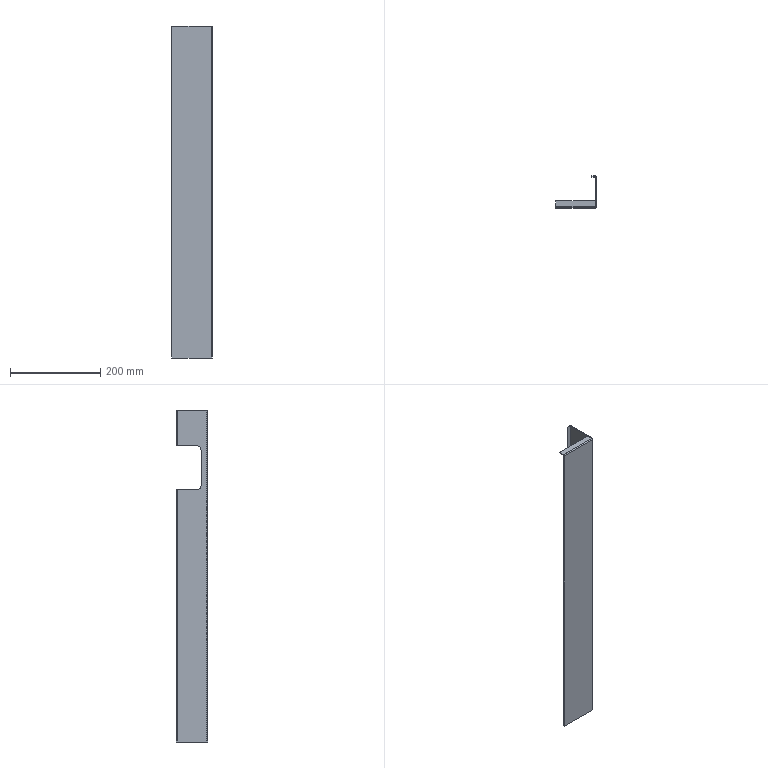Part | STEP file | Trunking 2 | 1 solid | 31 faces | box 90 x 70 x 735 mm | volume 175454 mm3 | plane 21 | cylinder 10 | commonest cylinder face diameters 1 x4 4 x4 20 x2
STEP:
#1=CARTESIAN_POINT('',(72.026,-9.818,0.));
#2=VERTEX_POINT('',#1);
#3=CARTESIAN_POINT('',(72.026,-9.818,733.));
#4=VERTEX_POINT('',#3);
#5=CARTESIAN_POINT('',(72.026,-9.818,735.));
#6=DIRECTION('',(0.,0.,1.));
#7=VECTOR('',#6,1000.);
#8=LINE('',#5,#7);
#9=EDGE_CURVE('',#2,#4,#8,.T.);
#10=ORIENTED_EDGE('',*,*,#9,.F.);
#11=CARTESIAN_POINT('',(-15.974,-9.818,0.));
#12=VERTEX_POINT('',#11);
#13=CARTESIAN_POINT('',(74.026,-9.818,0.));
#14=DIRECTION('',(1.,0.,0.));
#15=VECTOR('',#14,1000.);
#16=LINE('',#13,#15);
#17=EDGE_CURVE('',#12,#2,#16,.T.);
#18=ORIENTED_EDGE('',*,*,#17,.F.);
#19=CARTESIAN_POINT('',(-15.974,-9.818,733.));
#20=VERTEX_POINT('',#19);
#21=CARTESIAN_POINT('',(-15.974,-9.818,735.));
#22=DIRECTION('',(0.,0.,-1.));
#23=VECTOR('',#22,1000.);
#24=LINE('',#21,#23);
#25=EDGE_CURVE('',#20,#12,#24,.T.);
#26=ORIENTED_EDGE('',*,*,#25,.F.);
#27=CARTESIAN_POINT('',(74.026,-9.818,733.));
#28=DIRECTION('',(-1.,0.,0.));
#29=VECTOR('',#28,1000.);
#30=LINE('',#27,#29);
#31=EDGE_CURVE('',#4,#20,#30,.T.);
#32=ORIENTED_EDGE('',*,*,#31,.F.);
#33=EDGE_LOOP('',(#10,#18,#26,#32));
#34=FACE_OUTER_BOUND('',#33,.T.);
#35=CARTESIAN_POINT('',(74.026,-9.818,735.));
#36=DIRECTION('',(0.,-1.,0.));
#37=DIRECTION('',(1.,0.,0.));
#38=AXIS2_PLACEMENT_3D('',#35,#36,#37);
#39=PLANE('',#38);
#40=ADVANCED_FACE('',(#34),#39,.F.);
#41=CARTESIAN_POINT('',(-15.974,-9.318,733.5));
#42=VERTEX_POINT('',#41);
#43=CARTESIAN_POINT('',(-15.974,-9.318,733.));
#44=DIRECTION('',(1.,0.,0.));
#45=DIRECTION('',(0.,0.,-1.));
#46=AXIS2_PLACEMENT_3D('',#43,#44,#45);
#47=CIRCLE('',#46,0.5);
#48=EDGE_CURVE('',#42,#20,#47,.T.);
#49=ORIENTED_EDGE('',*,*,#48,.F.);
#50=CARTESIAN_POINT('',(72.026,-9.318,733.5));
#51=VERTEX_POINT('',#50);
#52=CARTESIAN_POINT('',(72.026,-9.318,733.5));
#53=DIRECTION('',(-1.,0.,0.));
#54=VECTOR('',#53,1000.);
#55=LINE('',#52,#54);
#56=EDGE_CURVE('',#51,#42,#55,.T.);
#57=ORIENTED_EDGE('',*,*,#56,.F.);
#58=CARTESIAN_POINT('',(72.026,-9.318,733.));
#59=DIRECTION('',(1.,0.,0.));
#60=DIRECTION('',(0.,0.,-1.));
#61=AXIS2_PLACEMENT_3D('',#58,#59,#60);
#62=CIRCLE('',#61,0.5);
#63=EDGE_CURVE('',#51,#4,#62,.T.);
#64=ORIENTED_EDGE('',*,*,#63,.T.);
#65=ORIENTED_EDGE('',*,*,#31,.T.);
#66=EDGE_LOOP('',(#49,#57,#64,#65));
#67=FACE_OUTER_BOUND('',#66,.T.);
#68=CARTESIAN_POINT('',(72.026,-9.318,733.));
#69=DIRECTION('',(1.,0.,0.));
#70=DIRECTION('',(0.,0.,-1.));
#71=AXIS2_PLACEMENT_3D('',#68,#69,#70);
#72=CYLINDRICAL_SURFACE('',#71,0.5);
#73=ADVANCED_FACE('',(#67),#72,.F.);
#74=ORIENTED_EDGE('',*,*,#9,.T.);
#75=CARTESIAN_POINT('',(72.026,-9.818,734.936));
#76=VERTEX_POINT('',#75);
#77=CARTESIAN_POINT('',(72.026,-9.818,735.));
#78=DIRECTION('',(0.,0.,-1.));
#79=VECTOR('',#78,1000.);
#80=LINE('',#77,#79);
#81=EDGE_CURVE('',#76,#4,#80,.T.);
#82=ORIENTED_EDGE('',*,*,#81,.F.);
#83=CARTESIAN_POINT('',(72.026,-9.818,735.));
#84=VERTEX_POINT('',#83);
#85=CARTESIAN_POINT('',(72.026,-9.818,735.));
#86=DIRECTION('',(0.,0.,-1.));
#87=VECTOR('',#86,1000.);
#88=LINE('',#85,#87);
#89=EDGE_CURVE('',#84,#76,#88,.T.);
#90=ORIENTED_EDGE('',*,*,#89,.F.);
#91=CARTESIAN_POINT('',(72.526,-9.318,735.));
#92=VERTEX_POINT('',#91);
#93=CARTESIAN_POINT('',(72.026,-9.318,735.));
#94=DIRECTION('',(0.,0.,-1.));
#95=DIRECTION('',(-1.,0.,0.));
#96=AXIS2_PLACEMENT_3D('',#93,#94,#95);
#97=CIRCLE('',#96,0.5);
#98=EDGE_CURVE('',#92,#84,#97,.T.);
#99=ORIENTED_EDGE('',*,*,#98,.F.);
#100=CARTESIAN_POINT('',(72.526,-9.318,0.));
#101=VERTEX_POINT('',#100);
#102=CARTESIAN_POINT('',(72.526,-9.318,735.));
#103=DIRECTION('',(0.,0.,1.));
#104=VECTOR('',#103,1000.);
#105=LINE('',#102,#104);
#106=EDGE_CURVE('',#101,#92,#105,.T.);
#107=ORIENTED_EDGE('',*,*,#106,.F.);
#108=CARTESIAN_POINT('',(72.026,-9.318,0.));
#109=DIRECTION('',(0.,0.,1.));
#110=DIRECTION('',(-1.,0.,0.));
#111=AXIS2_PLACEMENT_3D('',#108,#109,#110);
#112=CIRCLE('',#111,0.5);
#113=EDGE_CURVE('',#2,#101,#112,.T.);
#114=ORIENTED_EDGE('',*,*,#113,.F.);
#115=EDGE_LOOP('',(#74,#82,#90,#99,#107,#114));
#116=FACE_OUTER_BOUND('',#115,.T.);
#117=CARTESIAN_POINT('',(72.026,-9.318,735.));
#118=DIRECTION('',(0.,0.,-1.));
#119=DIRECTION('',(-1.,0.,0.));
#120=AXIS2_PLACEMENT_3D('',#117,#118,#119);
#121=CYLINDRICAL_SURFACE('',#120,0.5);
#122=ADVANCED_FACE('',(#116),#121,.F.);
#123=ORIENTED_EDGE('',*,*,#17,.T.);
#124=ORIENTED_EDGE('',*,*,#113,.T.);
#125=CARTESIAN_POINT('',(72.526,56.682,0.));
#126=VERTEX_POINT('',#125);
#127=CARTESIAN_POINT('',(72.526,58.682,0.));
#128=DIRECTION('',(0.,1.,0.));
#129=VECTOR('',#128,1000.);
#130=LINE('',#127,#129);
#131=EDGE_CURVE('',#101,#126,#130,.T.);
#132=ORIENTED_EDGE('',*,*,#131,.T.);
#133=CARTESIAN_POINT('',(72.026,57.182,0.));
#134=VERTEX_POINT('',#133);
#135=CARTESIAN_POINT('',(72.026,56.682,0.));
#136=DIRECTION('',(0.,0.,-1.));
#137=DIRECTION('',(-1.,0.,0.));
#138=AXIS2_PLACEMENT_3D('',#135,#136,#137);
#139=CIRCLE('',#138,0.5);
#140=EDGE_CURVE('',#134,#126,#139,.T.);
#141=ORIENTED_EDGE('',*,*,#140,.F.);
#142=CARTESIAN_POINT('',(64.026,57.182,0.));
#143=VERTEX_POINT('',#142);
#144=CARTESIAN_POINT('',(0.,57.182,0.));
#145=DIRECTION('',(1.,0.,0.));
#146=VECTOR('',#145,1000.);
#147=LINE('',#144,#146);
#148=EDGE_CURVE('',#143,#134,#147,.T.);
#149=ORIENTED_EDGE('',*,*,#148,.F.);
#150=CARTESIAN_POINT('',(64.026,58.682,0.));
#151=VERTEX_POINT('',#150);
#152=CARTESIAN_POINT('',(64.026,58.682,0.));
#153=DIRECTION('',(0.,1.,0.));
#154=VECTOR('',#153,1000.);
#155=LINE('',#152,#154);
#156=EDGE_CURVE('',#143,#151,#155,.T.);
#157=ORIENTED_EDGE('',*,*,#156,.T.);
#158=CARTESIAN_POINT('',(72.026,58.682,0.));
#159=VERTEX_POINT('',#158);
#160=CARTESIAN_POINT('',(0.,58.682,0.));
#161=DIRECTION('',(1.,0.,0.));
#162=VECTOR('',#161,1000.);
#163=LINE('',#160,#162);
#164=EDGE_CURVE('',#151,#159,#163,.T.);
#165=ORIENTED_EDGE('',*,*,#164,.T.);
#166=CARTESIAN_POINT('',(74.026,56.682,0.));
#167=VERTEX_POINT('',#166);
#168=CARTESIAN_POINT('',(72.026,56.682,0.));
#169=DIRECTION('',(0.,0.,1.));
#170=DIRECTION('',(-1.,0.,0.));
#171=AXIS2_PLACEMENT_3D('',#168,#169,#170);
#172=CIRCLE('',#171,2.);
#173=EDGE_CURVE('',#167,#159,#172,.T.);
#174=ORIENTED_EDGE('',*,*,#173,.F.);
#175=CARTESIAN_POINT('',(74.026,-9.318,0.));
#176=VERTEX_POINT('',#175);
#177=CARTESIAN_POINT('',(74.026,-9.818,0.));
#178=DIRECTION('',(0.,-1.,0.));
#179=VECTOR('',#178,1000.);
#180=LINE('',#177,#179);
#181=EDGE_CURVE('',#167,#176,#180,.T.);
#182=ORIENTED_EDGE('',*,*,#181,.T.);
#183=CARTESIAN_POINT('',(72.026,-11.318,0.));
#184=VERTEX_POINT('',#183);
#185=CARTESIAN_POINT('',(72.026,-9.318,0.));
#186=DIRECTION('',(0.,0.,1.));
#187=DIRECTION('',(-1.,0.,0.));
#188=AXIS2_PLACEMENT_3D('',#185,#186,#187);
#189=CIRCLE('',#188,2.);
#190=EDGE_CURVE('',#184,#176,#189,.T.);
#191=ORIENTED_EDGE('',*,*,#190,.F.);
#192=CARTESIAN_POINT('',(-15.974,-11.318,0.));
#193=VERTEX_POINT('',#192);
#194=CARTESIAN_POINT('',(72.026,-11.318,0.));
#195=DIRECTION('',(1.,0.,0.));
#196=VECTOR('',#195,1000.);
#197=LINE('',#194,#196);
#198=EDGE_CURVE('',#193,#184,#197,.T.);
#199=ORIENTED_EDGE('',*,*,#198,.F.);
#200=CARTESIAN_POINT('',(-15.974,-9.318,0.));
#201=DIRECTION('',(0.,-1.,0.));
#202=VECTOR('',#201,1000.);
#203=LINE('',#200,#202);
#204=EDGE_CURVE('',#12,#193,#203,.T.);
#205=ORIENTED_EDGE('',*,*,#204,.F.);
#206=EDGE_LOOP('',(#123,#124,#132,#141,#149,#157,#165,#174,#182,#191,#199,#205));
#207=FACE_OUTER_BOUND('',#206,.T.);
#208=CARTESIAN_POINT('',(72.026,-9.318,0.));
#209=DIRECTION('',(0.,0.,1.));
#210=DIRECTION('',(1.,0.,0.));
#211=AXIS2_PLACEMENT_3D('',#208,#209,#210);
#212=PLANE('',#211);
#213=ADVANCED_FACE('',(#207),#212,.F.);
#214=ORIENTED_EDGE('',*,*,#204,.T.);
#215=CARTESIAN_POINT('',(-15.974,-11.318,733.));
#216=VERTEX_POINT('',#215);
#217=CARTESIAN_POINT('',(-15.974,-11.318,735.));
#218=DIRECTION('',(0.,0.,1.));
#219=VECTOR('',#218,1000.);
#220=LINE('',#217,#219);
#221=EDGE_CURVE('',#193,#216,#220,.T.);
#222=ORIENTED_EDGE('',*,*,#221,.T.);
#223=CARTESIAN_POINT('',(-15.974,-9.318,735.));
#224=VERTEX_POINT('',#223);
#225=CARTESIAN_POINT('',(-15.974,-9.318,733.));
#226=DIRECTION('',(1.,0.,0.));
#227=DIRECTION('',(0.,0.,-1.));
#228=AXIS2_PLACEMENT_3D('',#225,#226,#227);
#229=CIRCLE('',#228,2.);
#230=EDGE_CURVE('',#224,#216,#229,.T.);
#231=ORIENTED_EDGE('',*,*,#230,.F.);
#232=CARTESIAN_POINT('',(-15.974,3.682,735.));
#233=VERTEX_POINT('',#232);
#234=CARTESIAN_POINT('',(-15.974,-9.818,735.));
#235=DIRECTION('',(0.,-1.,0.));
#236=VECTOR('',#235,1000.);
#237=LINE('',#234,#236);
#238=EDGE_CURVE('',#233,#224,#237,.T.);
#239=ORIENTED_EDGE('',*,*,#238,.F.);
#240=CARTESIAN_POINT('',(-15.974,3.682,733.5));
#241=VERTEX_POINT('',#240);
#242=CARTESIAN_POINT('',(-15.974,3.682,735.));
#243=DIRECTION('',(0.,0.,-1.));
#244=VECTOR('',#243,1000.);
#245=LINE('',#242,#244);
#246=EDGE_CURVE('',#233,#241,#245,.T.);
#247=ORIENTED_EDGE('',*,*,#246,.T.);
#248=CARTESIAN_POINT('',(-15.974,0.,733.5));
#249=DIRECTION('',(0.,1.,0.));
#250=VECTOR('',#249,1000.);
#251=LINE('',#248,#250);
#252=EDGE_CURVE('',#42,#241,#251,.T.);
#253=ORIENTED_EDGE('',*,*,#252,.F.);
#254=ORIENTED_EDGE('',*,*,#48,.T.);
#255=ORIENTED_EDGE('',*,*,#25,.T.);
#256=EDGE_LOOP('',(#214,#222,#231,#239,#247,#253,#254,#255));
#257=FACE_OUTER_BOUND('',#256,.T.);
#258=CARTESIAN_POINT('',(-15.974,-11.318,735.));
#259=DIRECTION('',(-1.,0.,0.));
#260=DIRECTION('',(0.,0.,1.));
#261=AXIS2_PLACEMENT_3D('',#258,#259,#260);
#262=PLANE('',#261);
#263=ADVANCED_FACE('',(#257),#262,.T.);
#264=ORIENTED_EDGE('',*,*,#252,.T.);
#265=CARTESIAN_POINT('',(72.026,3.682,733.5));
#266=VERTEX_POINT('',#265);
#267=CARTESIAN_POINT('',(0.,3.682,733.5));
#268=DIRECTION('',(1.,0.,0.));
#269=VECTOR('',#268,1000.);
#270=LINE('',#267,#269);
#271=EDGE_CURVE('',#241,#266,#270,.T.);
#272=ORIENTED_EDGE('',*,*,#271,.T.);
#273=CARTESIAN_POINT('',(72.026,0.,733.5));
#274=DIRECTION('',(0.,-1.,0.));
#275=VECTOR('',#274,1000.);
#276=LINE('',#273,#275);
#277=EDGE_CURVE('',#266,#51,#276,.T.);
#278=ORIENTED_EDGE('',*,*,#277,.T.);
#279=ORIENTED_EDGE('',*,*,#56,.T.);
#280=EDGE_LOOP('',(#264,#272,#278,#279));
#281=FACE_OUTER_BOUND('',#280,.T.);
#282=CARTESIAN_POINT('',(0.,0.,733.5));
#283=DIRECTION('',(0.,0.,-1.));
#284=DIRECTION('',(-1.,0.,0.));
#285=AXIS2_PLACEMENT_3D('',#282,#283,#284);
#286=PLANE('',#285);
#287=ADVANCED_FACE('',(#281),#286,.T.);
#288=ORIENTED_EDGE('',*,*,#81,.T.);
#289=ORIENTED_EDGE('',*,*,#63,.F.);
#290=ORIENTED_EDGE('',*,*,#277,.F.);
#291=CARTESIAN_POINT('',(72.026,3.682,735.));
#292=VERTEX_POINT('',#291);
#293=CARTESIAN_POINT('',(72.026,3.682,735.));
#294=DIRECTION('',(0.,0.,1.));
#295=VECTOR('',#294,1000.);
#296=LINE('',#293,#295);
#297=EDGE_CURVE('',#266,#292,#296,.T.);
#298=ORIENTED_EDGE('',*,*,#297,.T.);
#299=CARTESIAN_POINT('',(72.026,-9.318,735.));
#300=VERTEX_POINT('',#299);
#301=CARTESIAN_POINT('',(72.026,3.682,735.));
#302=DIRECTION('',(0.,1.,0.));
#303=VECTOR('',#302,1000.);
#304=LINE('',#301,#303);
#305=EDGE_CURVE('',#300,#292,#304,.T.);
#306=ORIENTED_EDGE('',*,*,#305,.F.);
#307=CARTESIAN_POINT('',(72.026,-9.318,733.));
#308=DIRECTION('',(-1.,0.,0.));
#309=DIRECTION('',(0.,0.,-1.));
#310=AXIS2_PLACEMENT_3D('',#307,#308,#309);
#311=CIRCLE('',#310,2.);
#312=EDGE_CURVE('',#76,#300,#311,.T.);
#313=ORIENTED_EDGE('',*,*,#312,.F.);
#314=EDGE_LOOP('',(#288,#289,#290,#298,#306,#313));
#315=FACE_OUTER_BOUND('',#314,.T.);
#316=CARTESIAN_POINT('',(72.026,-9.318,733.));
#317=DIRECTION('',(-1.,0.,0.));
#318=DIRECTION('',(0.,0.,1.));
#319=AXIS2_PLACEMENT_3D('',#316,#317,#318);
#320=PLANE('',#319);
#321=ADVANCED_FACE('',(#315),#320,.F.);
#322=CARTESIAN_POINT('',(72.526,13.682,656.));
#323=VERTEX_POINT('',#322);
#324=CARTESIAN_POINT('',(72.526,56.682,656.));
#325=VERTEX_POINT('',#324);
#326=CARTESIAN_POINT('',(72.526,58.682,656.));
#327=DIRECTION('',(0.,1.,0.));
#328=VECTOR('',#327,1000.);
#329=LINE('',#326,#328);
#330=EDGE_CURVE('',#323,#325,#329,.T.);
#331=ORIENTED_EDGE('',*,*,#330,.F.);
#332=CARTESIAN_POINT('',(72.526,3.682,646.));
#333=VERTEX_POINT('',#332);
#334=CARTESIAN_POINT('',(72.526,13.682,646.));
#335=DIRECTION('',(-1.,0.,0.));
#336=DIRECTION('',(0.,0.,-1.));
#337=AXIS2_PLACEMENT_3D('',#334,#335,#336);
#338=CIRCLE('',#337,10.);
#339=EDGE_CURVE('',#333,#323,#338,.T.);
#340=ORIENTED_EDGE('',*,*,#339,.F.);
#341=CARTESIAN_POINT('',(72.526,3.682,568.));
#342=VERTEX_POINT('',#341);
#343=CARTESIAN_POINT('',(72.526,3.682,735.));
#344=DIRECTION('',(0.,0.,1.));
#345=VECTOR('',#344,1000.);
#346=LINE('',#343,#345);
#347=EDGE_CURVE('',#342,#333,#346,.T.);
#348=ORIENTED_EDGE('',*,*,#347,.F.);
#349=CARTESIAN_POINT('',(72.526,13.682,558.));
#350=VERTEX_POINT('',#349);
#351=CARTESIAN_POINT('',(72.526,13.682,568.));
#352=DIRECTION('',(-1.,0.,0.));
#353=DIRECTION('',(0.,0.,-1.));
#354=AXIS2_PLACEMENT_3D('',#351,#352,#353);
#355=CIRCLE('',#354,10.);
#356=EDGE_CURVE('',#350,#342,#355,.T.);
#357=ORIENTED_EDGE('',*,*,#356,.F.);
#358=CARTESIAN_POINT('',(72.526,56.682,558.));
#359=VERTEX_POINT('',#358);
#360=CARTESIAN_POINT('',(72.526,58.682,558.));
#361=DIRECTION('',(0.,-1.,0.));
#362=VECTOR('',#361,1000.);
#363=LINE('',#360,#362);
#364=EDGE_CURVE('',#359,#350,#363,.T.);
#365=ORIENTED_EDGE('',*,*,#364,.F.);
#366=CARTESIAN_POINT('',(72.526,56.682,735.));
#367=DIRECTION('',(0.,0.,1.));
#368=VECTOR('',#367,1000.);
#369=LINE('',#366,#368);
#370=EDGE_CURVE('',#126,#359,#369,.T.);
#371=ORIENTED_EDGE('',*,*,#370,.F.);
#372=ORIENTED_EDGE('',*,*,#131,.F.);
#373=ORIENTED_EDGE('',*,*,#106,.T.);
#374=CARTESIAN_POINT('',(72.526,56.682,735.));
#375=VERTEX_POINT('',#374);
#376=CARTESIAN_POINT('',(72.526,58.682,735.));
#377=DIRECTION('',(0.,-1.,0.));
#378=VECTOR('',#377,1000.);
#379=LINE('',#376,#378);
#380=EDGE_CURVE('',#375,#92,#379,.T.);
#381=ORIENTED_EDGE('',*,*,#380,.F.);
#382=CARTESIAN_POINT('',(72.526,56.682,735.));
#383=DIRECTION('',(0.,0.,1.));
#384=VECTOR('',#383,1000.);
#385=LINE('',#382,#384);
#386=EDGE_CURVE('',#325,#375,#385,.T.);
#387=ORIENTED_EDGE('',*,*,#386,.F.);
#388=EDGE_LOOP('',(#331,#340,#348,#357,#365,#371,#372,#373,#381,#387));
#389=FACE_OUTER_BOUND('',#388,.T.);
#390=CARTESIAN_POINT('',(72.526,58.682,735.));
#391=DIRECTION('',(1.,0.,0.));
#392=DIRECTION('',(0.,0.,-1.));
#393=AXIS2_PLACEMENT_3D('',#390,#391,#392);
#394=PLANE('',#393);
#395=ADVANCED_FACE('',(#389),#394,.F.);
#396=ORIENTED_EDGE('',*,*,#221,.F.);
#397=ORIENTED_EDGE('',*,*,#198,.T.);
#398=CARTESIAN_POINT('',(72.026,-11.318,733.));
#399=VERTEX_POINT('',#398);
#400=CARTESIAN_POINT('',(72.026,-11.318,735.));
#401=DIRECTION('',(0.,0.,1.));
#402=VECTOR('',#401,1000.);
#403=LINE('',#400,#402);
#404=EDGE_CURVE('',#184,#399,#403,.T.);
#405=ORIENTED_EDGE('',*,*,#404,.T.);
#406=CARTESIAN_POINT('',(74.026,-11.318,733.));
#407=DIRECTION('',(-1.,0.,0.));
#408=VECTOR('',#407,1000.);
#409=LINE('',#406,#408);
#410=EDGE_CURVE('',#399,#216,#409,.T.);
#411=ORIENTED_EDGE('',*,*,#410,.T.);
#412=EDGE_LOOP('',(#396,#397,#405,#411));
#413=FACE_OUTER_BOUND('',#412,.T.);
#414=CARTESIAN_POINT('',(74.026,-11.318,735.));
#415=DIRECTION('',(0.,-1.,0.));
#416=DIRECTION('',(1.,0.,0.));
#417=AXIS2_PLACEMENT_3D('',#414,#415,#416);
#418=PLANE('',#417);
#419=ADVANCED_FACE('',(#413),#418,.T.);
#420=ORIENTED_EDGE('',*,*,#246,.F.);
#421=CARTESIAN_POINT('',(-15.974,3.682,735.));
#422=DIRECTION('',(-1.,0.,0.));
#423=VECTOR('',#422,1000.);
#424=LINE('',#421,#423);
#425=EDGE_CURVE('',#292,#233,#424,.T.);
#426=ORIENTED_EDGE('',*,*,#425,.F.);
#427=ORIENTED_EDGE('',*,*,#297,.F.);
#428=ORIENTED_EDGE('',*,*,#271,.F.);
#429=EDGE_LOOP('',(#420,#426,#427,#428));
#430=FACE_OUTER_BOUND('',#429,.T.);
#431=CARTESIAN_POINT('',(-15.974,3.682,735.));
#432=DIRECTION('',(0.,-1.,0.));
#433=DIRECTION('',(0.,0.,-1.));
#434=AXIS2_PLACEMENT_3D('',#431,#432,#433);
#435=PLANE('',#434);
#436=ADVANCED_FACE('',(#430),#435,.F.);
#437=CARTESIAN_POINT('',(72.026,57.182,656.));
#438=VERTEX_POINT('',#437);
#439=CARTESIAN_POINT('',(72.026,56.682,656.));
#440=DIRECTION('',(0.,0.,1.));
#441=DIRECTION('',(-1.,0.,0.));
#442=AXIS2_PLACEMENT_3D('',#439,#440,#441);
#443=CIRCLE('',#442,0.5);
#444=EDGE_CURVE('',#325,#438,#443,.T.);
#445=ORIENTED_EDGE('',*,*,#444,.F.);
#446=ORIENTED_EDGE('',*,*,#386,.T.);
#447=CARTESIAN_POINT('',(72.026,57.182,735.));
#448=VERTEX_POINT('',#447);
#449=CARTESIAN_POINT('',(72.026,56.682,735.));
#450=DIRECTION('',(0.,0.,-1.));
#451=DIRECTION('',(-1.,0.,0.));
#452=AXIS2_PLACEMENT_3D('',#449,#450,#451);
#453=CIRCLE('',#452,0.5);
#454=EDGE_CURVE('',#448,#375,#453,.T.);
#455=ORIENTED_EDGE('',*,*,#454,.F.);
#456=CARTESIAN_POINT('',(72.026,57.182,0.));
#457=DIRECTION('',(0.,0.,1.));
#458=VECTOR('',#457,1000.);
#459=LINE('',#456,#458);
#460=EDGE_CURVE('',#438,#448,#459,.T.);
#461=ORIENTED_EDGE('',*,*,#460,.F.);
#462=EDGE_LOOP('',(#445,#446,#455,#461));
#463=FACE_OUTER_BOUND('',#462,.T.);
#464=CARTESIAN_POINT('',(72.026,56.682,0.));
#465=DIRECTION('',(0.,0.,-1.));
#466=DIRECTION('',(-1.,0.,0.));
#467=AXIS2_PLACEMENT_3D('',#464,#465,#466);
#468=CYLINDRICAL_SURFACE('',#467,0.5);
#469=ADVANCED_FACE('',(#463),#468,.F.);
#470=CARTESIAN_POINT('',(74.026,13.682,656.));
#471=VERTEX_POINT('',#470);
#472=CARTESIAN_POINT('',(74.026,56.682,656.));
#473=VERTEX_POINT('',#472);
#474=CARTESIAN_POINT('',(74.026,58.682,656.));
#475=DIRECTION('',(0.,1.,0.));
#476=VECTOR('',#475,1000.);
#477=LINE('',#474,#476);
#478=EDGE_CURVE('',#471,#473,#477,.T.);
#479=ORIENTED_EDGE('',*,*,#478,.F.);
#480=CARTESIAN_POINT('',(64.026,13.682,656.));
#481=DIRECTION('',(1.,0.,0.));
#482=VECTOR('',#481,1000.);
#483=LINE('',#480,#482);
#484=EDGE_CURVE('',#323,#471,#483,.T.);
#485=ORIENTED_EDGE('',*,*,#484,.F.);
#486=ORIENTED_EDGE('',*,*,#330,.T.);
#487=ORIENTED_EDGE('',*,*,#444,.T.);
#488=CARTESIAN_POINT('',(64.026,57.182,656.));
#489=VERTEX_POINT('',#488);
#490=CARTESIAN_POINT('',(64.026,57.182,656.));
#491=DIRECTION('',(1.,0.,0.));
#492=VECTOR('',#491,1000.);
#493=LINE('',#490,#492);
#494=EDGE_CURVE('',#489,#438,#493,.T.);
#495=ORIENTED_EDGE('',*,*,#494,.F.);
#496=CARTESIAN_POINT('',(64.026,58.682,656.));
#497=VERTEX_POINT('',#496);
#498=CARTESIAN_POINT('',(64.026,58.682,656.));
#499=DIRECTION('',(0.,1.,0.));
#500=VECTOR('',#499,1000.);
#501=LINE('',#498,#500);
#502=EDGE_CURVE('',#489,#497,#501,.T.);
#503=ORIENTED_EDGE('',*,*,#502,.T.);
#504=CARTESIAN_POINT('',(72.026,58.682,656.));
#505=VERTEX_POINT('',#504);
#506=CARTESIAN_POINT('',(64.026,58.682,656.));
#507=DIRECTION('',(-1.,0.,0.));
#508=VECTOR('',#507,1000.);
#509=LINE('',#506,#508);
#510=EDGE_CURVE('',#505,#497,#509,.T.);
#511=ORIENTED_EDGE('',*,*,#510,.F.);
#512=CARTESIAN_POINT('',(72.026,56.682,656.));
#513=DIRECTION('',(0.,0.,1.));
#514=DIRECTION('',(-1.,0.,0.));
#515=AXIS2_PLACEMENT_3D('',#512,#513,#514);
#516=CIRCLE('',#515,2.);
#517=EDGE_CURVE('',#473,#505,#516,.T.);
#518=ORIENTED_EDGE('',*,*,#517,.F.);
#519=EDGE_LOOP('',(#479,#485,#486,#487,#495,#503,#511,#518));
#520=FACE_OUTER_BOUND('',#519,.T.);
#521=CARTESIAN_POINT('',(64.026,58.682,656.));
#522=DIRECTION('',(0.,0.,1.));
#523=DIRECTION('',(1.,0.,0.));
#524=AXIS2_PLACEMENT_3D('',#521,#522,#523);
#525=PLANE('',#524);
#526=ADVANCED_FACE('',(#520),#525,.F.);
#527=CARTESIAN_POINT('',(74.026,3.682,646.));
#528=VERTEX_POINT('',#527);
#529=CARTESIAN_POINT('',(74.026,13.682,646.));
#530=DIRECTION('',(-1.,0.,0.));
#531=DIRECTION('',(0.,0.,-1.));
#532=AXIS2_PLACEMENT_3D('',#529,#530,#531);
#533=CIRCLE('',#532,10.);
#534=EDGE_CURVE('',#528,#471,#533,.T.);
#535=ORIENTED_EDGE('',*,*,#534,.F.);
#536=CARTESIAN_POINT('',(64.026,3.682,646.));
#537=DIRECTION('',(1.,0.,0.));
#538=VECTOR('',#537,1000.);
#539=LINE('',#536,#538);
#540=EDGE_CURVE('',#333,#528,#539,.T.);
#541=ORIENTED_EDGE('',*,*,#540,.F.);
#542=ORIENTED_EDGE('',*,*,#339,.T.);
#543=ORIENTED_EDGE('',*,*,#484,.T.);
#544=EDGE_LOOP('',(#535,#541,#542,#543));
#545=FACE_OUTER_BOUND('',#544,.T.);
#546=CARTESIAN_POINT('',(64.026,13.682,646.));
#547=DIRECTION('',(1.,0.,0.));
#548=DIRECTION('',(0.,0.,-1.));
#549=AXIS2_PLACEMENT_3D('',#546,#547,#548);
#550=CYLINDRICAL_SURFACE('',#549,10.);
#551=ADVANCED_FACE('',(#545),#550,.F.);
#552=CARTESIAN_POINT('',(74.026,3.682,568.));
#553=VERTEX_POINT('',#552);
#554=CARTESIAN_POINT('',(74.026,3.682,646.));
#555=DIRECTION('',(0.,0.,1.));
#556=VECTOR('',#555,1000.);
#557=LINE('',#554,#556);
#558=EDGE_CURVE('',#553,#528,#557,.T.);
#559=ORIENTED_EDGE('',*,*,#558,.F.);
#560=CARTESIAN_POINT('',(64.026,3.682,568.));
#561=DIRECTION('',(1.,0.,0.));
#562=VECTOR('',#561,1000.);
#563=LINE('',#560,#562);
#564=EDGE_CURVE('',#342,#553,#563,.T.);
#565=ORIENTED_EDGE('',*,*,#564,.F.);
#566=ORIENTED_EDGE('',*,*,#347,.T.);
#567=ORIENTED_EDGE('',*,*,#540,.T.);
#568=EDGE_LOOP('',(#559,#565,#566,#567));
#569=FACE_OUTER_BOUND('',#568,.T.);
#570=CARTESIAN_POINT('',(64.026,3.682,646.));
#571=DIRECTION('',(0.,-1.,0.));
#572=DIRECTION('',(0.,0.,-1.));
#573=AXIS2_PLACEMENT_3D('',#570,#571,#572);
#574=PLANE('',#573);
#575=ADVANCED_FACE('',(#569),#574,.F.);
#576=CARTESIAN_POINT('',(74.026,13.682,558.));
#577=VERTEX_POINT('',#576);
#578=CARTESIAN_POINT('',(74.026,13.682,568.));
#579=DIRECTION('',(-1.,0.,0.));
#580=DIRECTION('',(0.,0.,-1.));
#581=AXIS2_PLACEMENT_3D('',#578,#579,#580);
#582=CIRCLE('',#581,10.);
#583=EDGE_CURVE('',#577,#553,#582,.T.);
#584=ORIENTED_EDGE('',*,*,#583,.F.);
#585=CARTESIAN_POINT('',(64.026,13.682,558.));
#586=DIRECTION('',(1.,0.,0.));
#587=VECTOR('',#586,1000.);
#588=LINE('',#585,#587);
#589=EDGE_CURVE('',#350,#577,#588,.T.);
#590=ORIENTED_EDGE('',*,*,#589,.F.);
#591=ORIENTED_EDGE('',*,*,#356,.T.);
#592=ORIENTED_EDGE('',*,*,#564,.T.);
#593=EDGE_LOOP('',(#584,#590,#591,#592));
#594=FACE_OUTER_BOUND('',#593,.T.);
#595=CARTESIAN_POINT('',(64.026,13.682,568.));
#596=DIRECTION('',(1.,0.,0.));
#597=DIRECTION('',(0.,0.,-1.));
#598=AXIS2_PLACEMENT_3D('',#595,#596,#597);
#599=CYLINDRICAL_SURFACE('',#598,10.);
#600=ADVANCED_FACE('',(#594),#599,.F.);
#601=CARTESIAN_POINT('',(64.026,58.682,558.));
#602=VERTEX_POINT('',#601);
#603=CARTESIAN_POINT('',(72.026,58.682,558.));
#604=VERTEX_POINT('',#603);
#605=CARTESIAN_POINT('',(64.026,58.682,558.));
#606=DIRECTION('',(1.,0.,0.));
#607=VECTOR('',#606,1000.);
#608=LINE('',#605,#607);
#609=EDGE_CURVE('',#602,#604,#608,.T.);
#610=ORIENTED_EDGE('',*,*,#609,.F.);
#611=CARTESIAN_POINT('',(64.026,57.182,558.));
#612=VERTEX_POINT('',#611);
#613=CARTESIAN_POINT('',(64.026,58.682,558.));
#614=DIRECTION('',(0.,-1.,0.));
#615=VECTOR('',#614,1000.);
#616=LINE('',#613,#615);
#617=EDGE_CURVE('',#602,#612,#616,.T.);
#618=ORIENTED_EDGE('',*,*,#617,.T.);
#619=CARTESIAN_POINT('',(72.026,57.182,558.));
#620=VERTEX_POINT('',#619);
#621=CARTESIAN_POINT('',(64.026,57.182,558.));
#622=DIRECTION('',(-1.,0.,0.));
#623=VECTOR('',#622,1000.);
#624=LINE('',#621,#623);
#625=EDGE_CURVE('',#620,#612,#624,.T.);
#626=ORIENTED_EDGE('',*,*,#625,.F.);
#627=CARTESIAN_POINT('',(72.026,56.682,558.));
#628=DIRECTION('',(0.,0.,1.));
#629=DIRECTION('',(-1.,0.,0.));
#630=AXIS2_PLACEMENT_3D('',#627,#628,#629);
#631=CIRCLE('',#630,0.5);
#632=EDGE_CURVE('',#359,#620,#631,.T.);
#633=ORIENTED_EDGE('',*,*,#632,.F.);
#634=ORIENTED_EDGE('',*,*,#364,.T.);
#635=ORIENTED_EDGE('',*,*,#589,.T.);
#636=CARTESIAN_POINT('',(74.026,56.682,558.));
#637=VERTEX_POINT('',#636);
#638=CARTESIAN_POINT('',(74.026,58.682,558.));
#639=DIRECTION('',(0.,-1.,0.));
#640=VECTOR('',#639,1000.);
#641=LINE('',#638,#640);
#642=EDGE_CURVE('',#637,#577,#641,.T.);
#643=ORIENTED_EDGE('',*,*,#642,.F.);
#644=CARTESIAN_POINT('',(72.026,56.682,558.));
#645=DIRECTION('',(0.,0.,-1.));
#646=DIRECTION('',(-1.,0.,0.));
#647=AXIS2_PLACEMENT_3D('',#644,#645,#646);
#648=CIRCLE('',#647,2.);
#649=EDGE_CURVE('',#604,#637,#648,.T.);
#650=ORIENTED_EDGE('',*,*,#649,.F.);
#651=EDGE_LOOP('',(#610,#618,#626,#633,#634,#635,#643,#650));
#652=FACE_OUTER_BOUND('',#651,.T.);
#653=CARTESIAN_POINT('',(64.026,58.682,558.));
#654=DIRECTION('',(0.,0.,-1.));
#655=DIRECTION('',(-1.,0.,0.));
#656=AXIS2_PLACEMENT_3D('',#653,#654,#655);
#657=PLANE('',#656);
#658=ADVANCED_FACE('',(#652),#657,.F.);
#659=ORIENTED_EDGE('',*,*,#632,.T.);
#660=CARTESIAN_POINT('',(72.026,57.182,0.));
#661=DIRECTION('',(0.,0.,1.));
#662=VECTOR('',#661,1000.);
#663=LINE('',#660,#662);
#664=EDGE_CURVE('',#134,#620,#663,.T.);
#665=ORIENTED_EDGE('',*,*,#664,.F.);
#666=ORIENTED_EDGE('',*,*,#140,.T.);
#667=ORIENTED_EDGE('',*,*,#370,.T.);
#668=EDGE_LOOP('',(#659,#665,#666,#667));
#669=FACE_OUTER_BOUND('',#668,.T.);
#670=CARTESIAN_POINT('',(72.026,56.682,0.));
#671=DIRECTION('',(0.,0.,-1.));
#672=DIRECTION('',(-1.,0.,0.));
#673=AXIS2_PLACEMENT_3D('',#670,#671,#672);
#674=CYLINDRICAL_SURFACE('',#673,0.5);
#675=ADVANCED_FACE('',(#669),#674,.F.);
#676=ORIENTED_EDGE('',*,*,#380,.T.);
#677=ORIENTED_EDGE('',*,*,#98,.T.);
#678=CARTESIAN_POINT('',(72.026,-11.318,735.));
#679=VERTEX_POINT('',#678);
#680=CARTESIAN_POINT('',(72.026,-9.818,735.));
#681=DIRECTION('',(0.,1.,0.));
#682=VECTOR('',#681,1000.);
#683=LINE('',#680,#682);
#684=EDGE_CURVE('',#679,#84,#683,.T.);
#685=ORIENTED_EDGE('',*,*,#684,.F.);
#686=CARTESIAN_POINT('',(74.026,-9.318,735.));
#687=VERTEX_POINT('',#686);
#688=CARTESIAN_POINT('',(72.026,-9.318,735.));
#689=DIRECTION('',(0.,0.,-1.));
#690=DIRECTION('',(-1.,0.,0.));
#691=AXIS2_PLACEMENT_3D('',#688,#689,#690);
#692=CIRCLE('',#691,2.);
#693=EDGE_CURVE('',#687,#679,#692,.T.);
#694=ORIENTED_EDGE('',*,*,#693,.F.);
#695=CARTESIAN_POINT('',(74.026,56.682,735.));
#696=VERTEX_POINT('',#695);
#697=CARTESIAN_POINT('',(74.026,-9.318,735.));
#698=DIRECTION('',(0.,1.,0.));
#699=VECTOR('',#698,1000.);
#700=LINE('',#697,#699);
#701=EDGE_CURVE('',#687,#696,#700,.T.);
#702=ORIENTED_EDGE('',*,*,#701,.T.);
#703=CARTESIAN_POINT('',(72.026,58.682,735.));
#704=VERTEX_POINT('',#703);
#705=CARTESIAN_POINT('',(72.026,56.682,735.));
#706=DIRECTION('',(0.,0.,-1.));
#707=DIRECTION('',(-1.,0.,0.));
#708=AXIS2_PLACEMENT_3D('',#705,#706,#707);
#709=CIRCLE('',#708,2.);
#710=EDGE_CURVE('',#704,#696,#709,.T.);
#711=ORIENTED_EDGE('',*,*,#710,.F.);
#712=CARTESIAN_POINT('',(64.026,58.682,735.));
#713=VERTEX_POINT('',#712);
#714=CARTESIAN_POINT('',(0.,58.682,735.));
#715=DIRECTION('',(-1.,0.,0.));
#716=VECTOR('',#715,1000.);
#717=LINE('',#714,#716);
#718=EDGE_CURVE('',#704,#713,#717,.T.);
#719=ORIENTED_EDGE('',*,*,#718,.T.);
#720=CARTESIAN_POINT('',(64.026,57.182,735.));
#721=VERTEX_POINT('',#720);
#722=CARTESIAN_POINT('',(64.026,58.682,735.));
#723=DIRECTION('',(0.,-1.,0.));
#724=VECTOR('',#723,1000.);
#725=LINE('',#722,#724);
#726=EDGE_CURVE('',#713,#721,#725,.T.);
#727=ORIENTED_EDGE('',*,*,#726,.T.);
#728=CARTESIAN_POINT('',(0.,57.182,735.));
#729=DIRECTION('',(-1.,0.,0.));
#730=VECTOR('',#729,1000.);
#731=LINE('',#728,#730);
#732=EDGE_CURVE('',#448,#721,#731,.T.);
#733=ORIENTED_EDGE('',*,*,#732,.F.);
#734=ORIENTED_EDGE('',*,*,#454,.T.);
#735=EDGE_LOOP('',(#676,#677,#685,#694,#702,#711,#719,#727,#733,#734));
#736=FACE_OUTER_BOUND('',#735,.T.);
#737=CARTESIAN_POINT('',(72.026,-9.318,735.));
#738=DIRECTION('',(0.,0.,1.));
#739=DIRECTION('',(1.,0.,0.));
#740=AXIS2_PLACEMENT_3D('',#737,#738,#739);
#741=PLANE('',#740);
#742=ADVANCED_FACE('',(#736),#741,.T.);
#743=CARTESIAN_POINT('',(72.026,-9.318,735.));
#744=DIRECTION('',(-1.,0.,0.));
#745=VECTOR('',#744,1000.);
#746=LINE('',#743,#745);
#747=EDGE_CURVE('',#300,#224,#746,.T.);
#748=ORIENTED_EDGE('',*,*,#747,.T.);
#749=ORIENTED_EDGE('',*,*,#230,.T.);
#750=ORIENTED_EDGE('',*,*,#410,.F.);
#751=CARTESIAN_POINT('',(72.026,-9.318,733.));
#752=DIRECTION('',(-1.,0.,0.));
#753=DIRECTION('',(0.,0.,-1.));
#754=AXIS2_PLACEMENT_3D('',#751,#752,#753);
#755=CIRCLE('',#754,2.);
#756=EDGE_CURVE('',#399,#76,#755,.T.);
#757=ORIENTED_EDGE('',*,*,#756,.T.);
#758=ORIENTED_EDGE('',*,*,#312,.T.);
#759=EDGE_LOOP('',(#748,#749,#750,#757,#758));
#760=FACE_OUTER_BOUND('',#759,.T.);
#761=CARTESIAN_POINT('',(72.026,-9.318,733.));
#762=DIRECTION('',(1.,0.,0.));
#763=DIRECTION('',(0.,0.,-1.));
#764=AXIS2_PLACEMENT_3D('',#761,#762,#763);
#765=CYLINDRICAL_SURFACE('',#764,2.);
#766=ADVANCED_FACE('',(#760),#765,.T.);
#767=CARTESIAN_POINT('',(72.026,-11.318,735.));
#768=DIRECTION('',(0.,0.,-1.));
#769=VECTOR('',#768,1000.);
#770=LINE('',#767,#769);
#771=EDGE_CURVE('',#679,#399,#770,.T.);
#772=ORIENTED_EDGE('',*,*,#771,.T.);
#773=ORIENTED_EDGE('',*,*,#404,.F.);
#774=ORIENTED_EDGE('',*,*,#190,.T.);
#775=CARTESIAN_POINT('',(74.026,-9.318,735.));
#776=DIRECTION('',(0.,0.,1.));
#777=VECTOR('',#776,1000.);
#778=LINE('',#775,#777);
#779=EDGE_CURVE('',#176,#687,#778,.T.);
#780=ORIENTED_EDGE('',*,*,#779,.T.);
#781=ORIENTED_EDGE('',*,*,#693,.T.);
#782=EDGE_LOOP('',(#772,#773,#774,#780,#781));
#783=FACE_OUTER_BOUND('',#782,.T.);
#784=CARTESIAN_POINT('',(72.026,-9.318,735.));
#785=DIRECTION('',(0.,0.,-1.));
#786=DIRECTION('',(-1.,0.,0.));
#787=AXIS2_PLACEMENT_3D('',#784,#785,#786);
#788=CYLINDRICAL_SURFACE('',#787,2.);
#789=ADVANCED_FACE('',(#783),#788,.T.);
#790=ORIENTED_EDGE('',*,*,#305,.T.);
#791=ORIENTED_EDGE('',*,*,#425,.T.);
#792=ORIENTED_EDGE('',*,*,#238,.T.);
#793=ORIENTED_EDGE('',*,*,#747,.F.);
#794=EDGE_LOOP('',(#790,#791,#792,#793));
#795=FACE_OUTER_BOUND('',#794,.T.);
#796=CARTESIAN_POINT('',(0.,0.,735.));
#797=DIRECTION('',(0.,0.,-1.));
#798=DIRECTION('',(-1.,0.,0.));
#799=AXIS2_PLACEMENT_3D('',#796,#797,#798);
#800=PLANE('',#799);
#801=ADVANCED_FACE('',(#795),#800,.F.);
#802=ORIENTED_EDGE('',*,*,#732,.T.);
#803=CARTESIAN_POINT('',(64.026,57.182,0.));
#804=DIRECTION('',(0.,0.,-1.));
#805=VECTOR('',#804,1000.);
#806=LINE('',#803,#805);
#807=EDGE_CURVE('',#721,#489,#806,.T.);
#808=ORIENTED_EDGE('',*,*,#807,.T.);
#809=ORIENTED_EDGE('',*,*,#494,.T.);
#810=ORIENTED_EDGE('',*,*,#460,.T.);
#811=EDGE_LOOP('',(#802,#808,#809,#810));
#812=FACE_OUTER_BOUND('',#811,.T.);
#813=CARTESIAN_POINT('',(0.,57.182,0.));
#814=DIRECTION('',(0.,-1.,0.));
#815=DIRECTION('',(1.,0.,0.));
#816=AXIS2_PLACEMENT_3D('',#813,#814,#815);
#817=PLANE('',#816);
#818=ADVANCED_FACE('',(#812),#817,.T.);
#819=ORIENTED_EDGE('',*,*,#710,.T.);
#820=CARTESIAN_POINT('',(74.026,56.682,0.));
#821=DIRECTION('',(0.,0.,-1.));
#822=VECTOR('',#821,1000.);
#823=LINE('',#820,#822);
#824=EDGE_CURVE('',#696,#473,#823,.T.);
#825=ORIENTED_EDGE('',*,*,#824,.T.);
#826=ORIENTED_EDGE('',*,*,#517,.T.);
#827=CARTESIAN_POINT('',(72.026,58.682,0.));
#828=DIRECTION('',(0.,0.,1.));
#829=VECTOR('',#828,1000.);
#830=LINE('',#827,#829);
#831=EDGE_CURVE('',#505,#704,#830,.T.);
#832=ORIENTED_EDGE('',*,*,#831,.T.);
#833=EDGE_LOOP('',(#819,#825,#826,#832));
#834=FACE_OUTER_BOUND('',#833,.T.);
#835=CARTESIAN_POINT('',(72.026,56.682,0.));
#836=DIRECTION('',(0.,0.,-1.));
#837=DIRECTION('',(-1.,0.,0.));
#838=AXIS2_PLACEMENT_3D('',#835,#836,#837);
#839=CYLINDRICAL_SURFACE('',#838,2.);
#840=ADVANCED_FACE('',(#834),#839,.T.);
#841=ORIENTED_EDGE('',*,*,#558,.T.);
#842=ORIENTED_EDGE('',*,*,#534,.T.);
#843=ORIENTED_EDGE('',*,*,#478,.T.);
#844=ORIENTED_EDGE('',*,*,#824,.F.);
#845=ORIENTED_EDGE('',*,*,#701,.F.);
#846=ORIENTED_EDGE('',*,*,#779,.F.);
#847=ORIENTED_EDGE('',*,*,#181,.F.);
#848=CARTESIAN_POINT('',(74.026,56.682,735.));
#849=DIRECTION('',(0.,0.,1.));
#850=VECTOR('',#849,1000.);
#851=LINE('',#848,#850);
#852=EDGE_CURVE('',#167,#637,#851,.T.);
#853=ORIENTED_EDGE('',*,*,#852,.T.);
#854=ORIENTED_EDGE('',*,*,#642,.T.);
#855=ORIENTED_EDGE('',*,*,#583,.T.);
#856=EDGE_LOOP('',(#841,#842,#843,#844,#845,#846,#847,#853,#854,#855));
#857=FACE_OUTER_BOUND('',#856,.T.);
#858=CARTESIAN_POINT('',(74.026,58.682,735.));
#859=DIRECTION('',(1.,0.,0.));
#860=DIRECTION('',(0.,0.,-1.));
#861=AXIS2_PLACEMENT_3D('',#858,#859,#860);
#862=PLANE('',#861);
#863=ADVANCED_FACE('',(#857),#862,.T.);
#864=ORIENTED_EDGE('',*,*,#510,.T.);
#865=CARTESIAN_POINT('',(64.026,58.682,0.));
#866=DIRECTION('',(0.,0.,-1.));
#867=VECTOR('',#866,1000.);
#868=LINE('',#865,#867);
#869=EDGE_CURVE('',#713,#497,#868,.T.);
#870=ORIENTED_EDGE('',*,*,#869,.F.);
#871=ORIENTED_EDGE('',*,*,#718,.F.);
#872=ORIENTED_EDGE('',*,*,#831,.F.);
#873=EDGE_LOOP('',(#864,#870,#871,#872));
#874=FACE_OUTER_BOUND('',#873,.T.);
#875=CARTESIAN_POINT('',(0.,58.682,0.));
#876=DIRECTION('',(0.,-1.,0.));
#877=DIRECTION('',(1.,0.,0.));
#878=AXIS2_PLACEMENT_3D('',#875,#876,#877);
#879=PLANE('',#878);
#880=ADVANCED_FACE('',(#874),#879,.F.);
#881=ORIENTED_EDGE('',*,*,#173,.T.);
#882=CARTESIAN_POINT('',(72.026,58.682,0.));
#883=DIRECTION('',(0.,0.,1.));
#884=VECTOR('',#883,1000.);
#885=LINE('',#882,#884);
#886=EDGE_CURVE('',#159,#604,#885,.T.);
#887=ORIENTED_EDGE('',*,*,#886,.T.);
#888=ORIENTED_EDGE('',*,*,#649,.T.);
#889=ORIENTED_EDGE('',*,*,#852,.F.);
#890=EDGE_LOOP('',(#881,#887,#888,#889));
#891=FACE_OUTER_BOUND('',#890,.T.);
#892=CARTESIAN_POINT('',(72.026,56.682,0.));
#893=DIRECTION('',(0.,0.,-1.));
#894=DIRECTION('',(-1.,0.,0.));
#895=AXIS2_PLACEMENT_3D('',#892,#893,#894);
#896=CYLINDRICAL_SURFACE('',#895,2.);
#897=ADVANCED_FACE('',(#891),#896,.T.);
#898=ORIENTED_EDGE('',*,*,#609,.T.);
#899=ORIENTED_EDGE('',*,*,#886,.F.);
#900=ORIENTED_EDGE('',*,*,#164,.F.);
#901=CARTESIAN_POINT('',(64.026,58.682,0.));
#902=DIRECTION('',(0.,0.,-1.));
#903=VECTOR('',#902,1000.);
#904=LINE('',#901,#903);
#905=EDGE_CURVE('',#602,#151,#904,.T.);
#906=ORIENTED_EDGE('',*,*,#905,.F.);
#907=EDGE_LOOP('',(#898,#899,#900,#906));
#908=FACE_OUTER_BOUND('',#907,.T.);
#909=CARTESIAN_POINT('',(0.,58.682,0.));
#910=DIRECTION('',(0.,-1.,0.));
#911=DIRECTION('',(1.,0.,0.));
#912=AXIS2_PLACEMENT_3D('',#909,#910,#911);
#913=PLANE('',#912);
#914=ADVANCED_FACE('',(#908),#913,.F.);
#915=ORIENTED_EDGE('',*,*,#148,.T.);
#916=ORIENTED_EDGE('',*,*,#664,.T.);
#917=ORIENTED_EDGE('',*,*,#625,.T.);
#918=CARTESIAN_POINT('',(64.026,57.182,0.));
#919=DIRECTION('',(0.,0.,-1.));
#920=VECTOR('',#919,1000.);
#921=LINE('',#918,#920);
#922=EDGE_CURVE('',#612,#143,#921,.T.);
#923=ORIENTED_EDGE('',*,*,#922,.T.);
#924=EDGE_LOOP('',(#915,#916,#917,#923));
#925=FACE_OUTER_BOUND('',#924,.T.);
#926=CARTESIAN_POINT('',(0.,57.182,0.));
#927=DIRECTION('',(0.,-1.,0.));
#928=DIRECTION('',(1.,0.,0.));
#929=AXIS2_PLACEMENT_3D('',#926,#927,#928);
#930=PLANE('',#929);
#931=ADVANCED_FACE('',(#925),#930,.T.);
#932=ORIENTED_EDGE('',*,*,#771,.F.);
#933=ORIENTED_EDGE('',*,*,#684,.T.);
#934=ORIENTED_EDGE('',*,*,#89,.T.);
#935=ORIENTED_EDGE('',*,*,#756,.F.);
#936=EDGE_LOOP('',(#932,#933,#934,#935));
#937=FACE_OUTER_BOUND('',#936,.T.);
#938=CARTESIAN_POINT('',(72.026,-9.818,735.));
#939=DIRECTION('',(-1.,0.,0.));
#940=DIRECTION('',(0.,-1.,0.));
#941=AXIS2_PLACEMENT_3D('',#938,#939,#940);
#942=PLANE('',#941);
#943=ADVANCED_FACE('',(#937),#942,.T.);
#944=ORIENTED_EDGE('',*,*,#502,.F.);
#945=ORIENTED_EDGE('',*,*,#807,.F.);
#946=ORIENTED_EDGE('',*,*,#726,.F.);
#947=ORIENTED_EDGE('',*,*,#869,.T.);
#948=EDGE_LOOP('',(#944,#945,#946,#947));
#949=FACE_OUTER_BOUND('',#948,.T.);
#950=CARTESIAN_POINT('',(64.026,58.682,735.));
#951=DIRECTION('',(1.,0.,0.));
#952=DIRECTION('',(0.,1.,0.));
#953=AXIS2_PLACEMENT_3D('',#950,#951,#952);
#954=PLANE('',#953);
#955=ADVANCED_FACE('',(#949),#954,.F.);
#956=ORIENTED_EDGE('',*,*,#617,.F.);
#957=ORIENTED_EDGE('',*,*,#905,.T.);
#958=ORIENTED_EDGE('',*,*,#156,.F.);
#959=ORIENTED_EDGE('',*,*,#922,.F.);
#960=EDGE_LOOP('',(#956,#957,#958,#959));
#961=FACE_OUTER_BOUND('',#960,.T.);
#962=CARTESIAN_POINT('',(64.026,58.682,735.));
#963=DIRECTION('',(1.,0.,0.));
#964=DIRECTION('',(0.,1.,0.));
#965=AXIS2_PLACEMENT_3D('',#962,#963,#964);
#966=PLANE('',#965);
#967=ADVANCED_FACE('',(#961),#966,.F.);
#968=CLOSED_SHELL('',(#40,#73,#122,#213,#263,#287,#321,#395,#419,#436,#469,#526,#551,#575,#600,#658,#675,#742,#766,#789,#801,#818,#840,#863,#880,#897,#914,#931,#943,#955,#967));
#969=MANIFOLD_SOLID_BREP('',#968);
#970=CARTESIAN_POINT('',(0.,0.,0.));
#971=DIRECTION('',(0.,0.,1.));
#972=DIRECTION('',(1.,0.,0.));
#973=AXIS2_PLACEMENT_3D('',#970,#971,#972);
#974=(LENGTH_UNIT()NAMED_UNIT(*)SI_UNIT(.MILLI.,.METRE.));
#975=UNCERTAINTY_MEASURE_WITH_UNIT(LENGTH_MEASURE(0.00001),#974,'','');
#976=(NAMED_UNIT(*)PLANE_ANGLE_UNIT()SI_UNIT($,.RADIAN.));
#977=(NAMED_UNIT(*)SI_UNIT($,.STERADIAN.)SOLID_ANGLE_UNIT());
#978=(GEOMETRIC_REPRESENTATION_CONTEXT(3)GLOBAL_UNCERTAINTY_ASSIGNED_CONTEXT((#975))GLOBAL_UNIT_ASSIGNED_CONTEXT((#974,#976,#977))REPRESENTATION_CONTEXT('',''));
#979=ADVANCED_BREP_SHAPE_REPRESENTATION('',(#969,#973),#978);